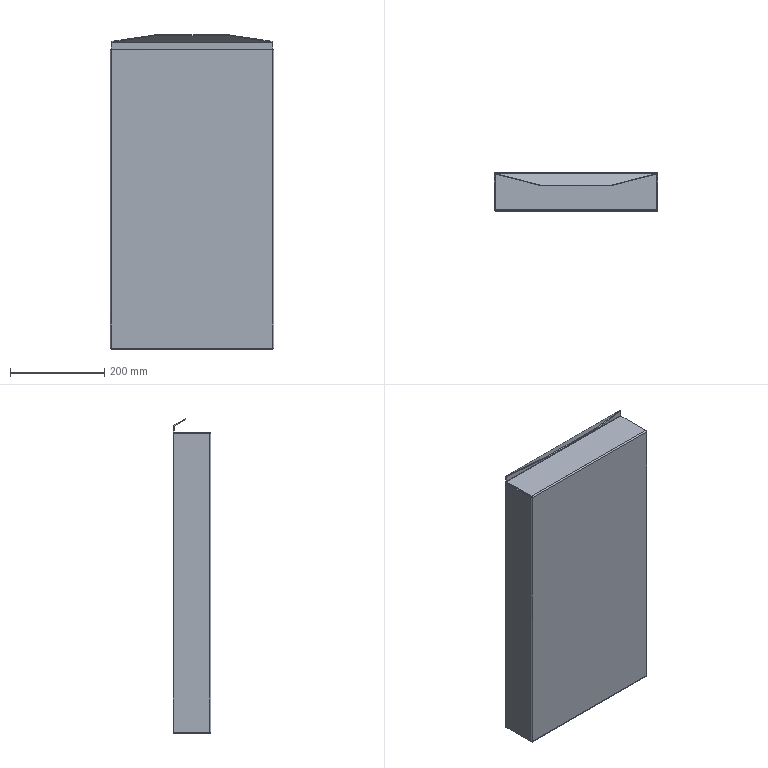Part | SolidWorks | features EdgeFlange 3, FlatPattern 1, ICE 1, SMBaseFlange 1, SheetMetal 1 | 1 solid | 54 faces | box 348 x 80 x 668.155 mm | volume 769690 mm3 | plane 34 | cylinder 12 | spline 8 | commonest cylinder face diameters 1.473 x6 5.473 x6